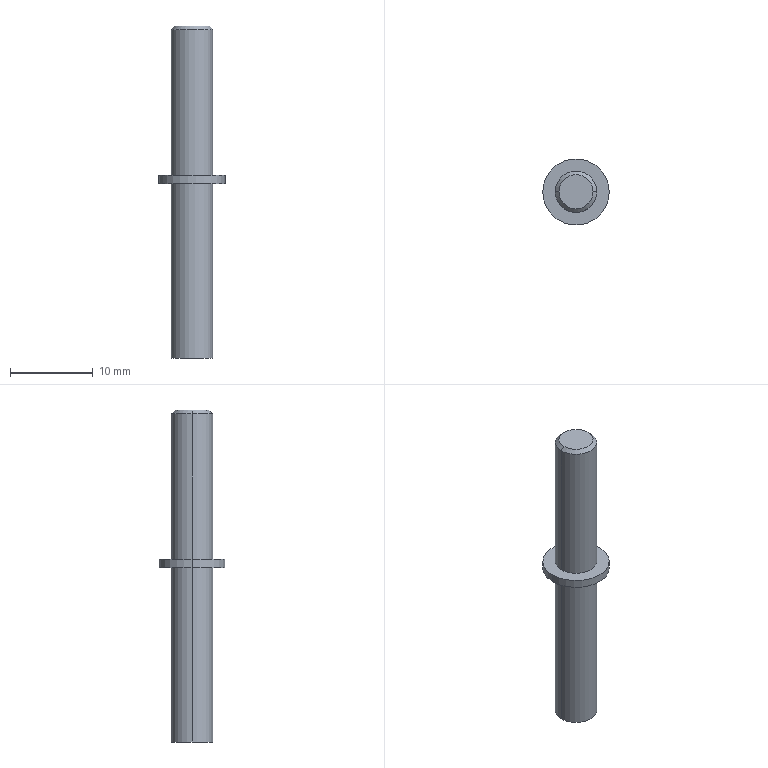Part | SolidWorks | features ICE 2, 3DProfileFeature 1, Extrusion 1, HoleWzd 1, StudWizard 1 | 1 solid | 16 faces | box 8 x 8 x 40 mm | volume 765.722 mm3 | cylinder 8 | cone 4 | plane 4 | commonest cylinder face diameters 5 x4 2.5 x2 8 x2
STEP:
#1=CARTESIAN_POINT('',(0.,0.,-10.549));
#2=VERTEX_POINT('',#1);
#3=CARTESIAN_POINT('',(-1.25,0.,-11.3));
#4=VERTEX_POINT('',#3);
#5=CARTESIAN_POINT('',(-1.25,0.,-11.3));
#6=DIRECTION('',(-0.8572,0.,-0.515));
#7=VECTOR('',#6,1000.);
#8=LINE('',#5,#7);
#9=EDGE_CURVE('',#2,#4,#8,.T.);
#10=ORIENTED_EDGE('',*,*,#9,.F.);
#11=CARTESIAN_POINT('',(1.25,0.,-11.3));
#12=VERTEX_POINT('',#11);
#13=CARTESIAN_POINT('',(1.25,0.,-11.3));
#14=DIRECTION('',(0.8572,0.,-0.515));
#15=VECTOR('',#14,1000.);
#16=LINE('',#13,#15);
#17=EDGE_CURVE('',#2,#12,#16,.T.);
#18=ORIENTED_EDGE('',*,*,#17,.T.);
#19=CARTESIAN_POINT('',(0.,0.,-11.3));
#20=DIRECTION('',(0.,0.,-1.));
#21=DIRECTION('',(-1.,0.,0.));
#22=AXIS2_PLACEMENT_3D('',#19,#20,#21);
#23=CIRCLE('',#22,1.25);
#24=EDGE_CURVE('',#12,#4,#23,.T.);
#25=ORIENTED_EDGE('',*,*,#24,.T.);
#26=EDGE_LOOP('',(#10,#18,#25));
#27=FACE_OUTER_BOUND('',#26,.T.);
#28=CARTESIAN_POINT('',(0.,0.,-11.3));
#29=DIRECTION('',(0.,0.,-1.));
#30=DIRECTION('',(-1.,0.,0.));
#31=AXIS2_PLACEMENT_3D('',#28,#29,#30);
#32=CONICAL_SURFACE('',#31,1.25,1.03);
#33=ADVANCED_FACE('',(#27),#32,.F.);
#34=ORIENTED_EDGE('',*,*,#24,.F.);
#35=CARTESIAN_POINT('',(1.25,0.,-21.));
#36=VERTEX_POINT('',#35);
#37=CARTESIAN_POINT('',(1.25,0.,-21.3));
#38=DIRECTION('',(0.,0.,-1.));
#39=VECTOR('',#38,1000.);
#40=LINE('',#37,#39);
#41=EDGE_CURVE('',#12,#36,#40,.T.);
#42=ORIENTED_EDGE('',*,*,#41,.T.);
#43=CARTESIAN_POINT('',(-1.25,0.,-21.));
#44=VERTEX_POINT('',#43);
#45=CARTESIAN_POINT('',(0.,0.,-21.));
#46=DIRECTION('',(0.,0.,1.));
#47=DIRECTION('',(1.,0.,0.));
#48=AXIS2_PLACEMENT_3D('',#45,#46,#47);
#49=CIRCLE('',#48,1.25);
#50=EDGE_CURVE('',#44,#36,#49,.T.);
#51=ORIENTED_EDGE('',*,*,#50,.F.);
#52=CARTESIAN_POINT('',(-1.25,0.,-21.3));
#53=DIRECTION('',(0.,0.,-1.));
#54=VECTOR('',#53,1000.);
#55=LINE('',#52,#54);
#56=EDGE_CURVE('',#4,#44,#55,.T.);
#57=ORIENTED_EDGE('',*,*,#56,.F.);
#58=EDGE_LOOP('',(#34,#42,#51,#57));
#59=FACE_OUTER_BOUND('',#58,.T.);
#60=CARTESIAN_POINT('',(0.,0.,-21.3));
#61=DIRECTION('',(0.,0.,-1.));
#62=DIRECTION('',(-1.,0.,0.));
#63=AXIS2_PLACEMENT_3D('',#60,#61,#62);
#64=CYLINDRICAL_SURFACE('',#63,1.25);
#65=ADVANCED_FACE('',(#59),#64,.F.);
#66=CARTESIAN_POINT('',(-2.055,0.,19.));
#67=VERTEX_POINT('',#66);
#68=CARTESIAN_POINT('',(2.055,0.,19.));
#69=VERTEX_POINT('',#68);
#70=CARTESIAN_POINT('',(0.,0.,19.));
#71=DIRECTION('',(0.,0.,-1.));
#72=DIRECTION('',(-1.,0.,0.));
#73=AXIS2_PLACEMENT_3D('',#70,#71,#72);
#74=CIRCLE('',#73,2.055);
#75=EDGE_CURVE('',#67,#69,#74,.T.);
#76=ORIENTED_EDGE('',*,*,#75,.T.);
#77=CARTESIAN_POINT('',(2.5,0.,18.555));
#78=VERTEX_POINT('',#77);
#79=CARTESIAN_POINT('',(2.055,0.,19.));
#80=DIRECTION('',(0.7071,0.,-0.7071));
#81=VECTOR('',#80,1000.);
#82=LINE('',#79,#81);
#83=EDGE_CURVE('',#69,#78,#82,.T.);
#84=ORIENTED_EDGE('',*,*,#83,.T.);
#85=CARTESIAN_POINT('',(-2.5,0.,18.555));
#86=VERTEX_POINT('',#85);
#87=CARTESIAN_POINT('',(0.,0.,18.555));
#88=DIRECTION('',(0.,0.,-1.));
#89=DIRECTION('',(-1.,0.,0.));
#90=AXIS2_PLACEMENT_3D('',#87,#88,#89);
#91=CIRCLE('',#90,2.5);
#92=EDGE_CURVE('',#86,#78,#91,.T.);
#93=ORIENTED_EDGE('',*,*,#92,.F.);
#94=CARTESIAN_POINT('',(-2.055,0.,19.));
#95=DIRECTION('',(-0.7071,0.,-0.7071));
#96=VECTOR('',#95,1000.);
#97=LINE('',#94,#96);
#98=EDGE_CURVE('',#67,#86,#97,.T.);
#99=ORIENTED_EDGE('',*,*,#98,.F.);
#100=EDGE_LOOP('',(#76,#84,#93,#99));
#101=FACE_OUTER_BOUND('',#100,.T.);
#102=CARTESIAN_POINT('',(0.,0.,19.));
#103=DIRECTION('',(0.,0.,-1.));
#104=DIRECTION('',(-1.,0.,0.));
#105=AXIS2_PLACEMENT_3D('',#102,#103,#104);
#106=CONICAL_SURFACE('',#105,2.055,0.7854);
#107=ADVANCED_FACE('',(#101),#106,.T.);
#108=ORIENTED_EDGE('',*,*,#92,.T.);
#109=CARTESIAN_POINT('',(2.5,0.,1.));
#110=VERTEX_POINT('',#109);
#111=CARTESIAN_POINT('',(2.5,0.,19.));
#112=DIRECTION('',(0.,0.,-1.));
#113=VECTOR('',#112,1000.);
#114=LINE('',#111,#113);
#115=EDGE_CURVE('',#78,#110,#114,.T.);
#116=ORIENTED_EDGE('',*,*,#115,.T.);
#117=CARTESIAN_POINT('',(-2.5,0.,1.));
#118=VERTEX_POINT('',#117);
#119=CARTESIAN_POINT('',(0.,0.,1.));
#120=DIRECTION('',(0.,0.,1.));
#121=DIRECTION('',(1.,0.,0.));
#122=AXIS2_PLACEMENT_3D('',#119,#120,#121);
#123=CIRCLE('',#122,2.5);
#124=EDGE_CURVE('',#110,#118,#123,.T.);
#125=ORIENTED_EDGE('',*,*,#124,.T.);
#126=CARTESIAN_POINT('',(-2.5,0.,19.));
#127=DIRECTION('',(0.,0.,-1.));
#128=VECTOR('',#127,1000.);
#129=LINE('',#126,#128);
#130=EDGE_CURVE('',#86,#118,#129,.T.);
#131=ORIENTED_EDGE('',*,*,#130,.F.);
#132=EDGE_LOOP('',(#108,#116,#125,#131));
#133=FACE_OUTER_BOUND('',#132,.T.);
#134=CARTESIAN_POINT('',(0.,0.,19.));
#135=DIRECTION('',(0.,0.,-1.));
#136=DIRECTION('',(-1.,0.,0.));
#137=AXIS2_PLACEMENT_3D('',#134,#135,#136);
#138=CYLINDRICAL_SURFACE('',#137,2.5);
#139=ADVANCED_FACE('',(#133),#138,.T.);
#140=CARTESIAN_POINT('',(4.,0.,1.));
#141=VERTEX_POINT('',#140);
#142=CARTESIAN_POINT('',(-4.,0.,1.));
#143=VERTEX_POINT('',#142);
#144=CARTESIAN_POINT('',(0.,0.,1.));
#145=DIRECTION('',(0.,0.,1.));
#146=DIRECTION('',(1.,0.,0.));
#147=AXIS2_PLACEMENT_3D('',#144,#145,#146);
#148=CIRCLE('',#147,4.);
#149=EDGE_CURVE('',#141,#143,#148,.T.);
#150=ORIENTED_EDGE('',*,*,#149,.F.);
#151=CARTESIAN_POINT('',(4.,0.,0.));
#152=VERTEX_POINT('',#151);
#153=CARTESIAN_POINT('',(4.,0.,1.));
#154=DIRECTION('',(0.,0.,-1.));
#155=VECTOR('',#154,1000.);
#156=LINE('',#153,#155);
#157=EDGE_CURVE('',#141,#152,#156,.T.);
#158=ORIENTED_EDGE('',*,*,#157,.T.);
#159=CARTESIAN_POINT('',(-4.,0.,0.));
#160=VERTEX_POINT('',#159);
#161=CARTESIAN_POINT('',(0.,0.,0.));
#162=DIRECTION('',(0.,0.,1.));
#163=DIRECTION('',(1.,0.,0.));
#164=AXIS2_PLACEMENT_3D('',#161,#162,#163);
#165=CIRCLE('',#164,4.);
#166=EDGE_CURVE('',#152,#160,#165,.T.);
#167=ORIENTED_EDGE('',*,*,#166,.T.);
#168=CARTESIAN_POINT('',(-4.,0.,1.));
#169=DIRECTION('',(0.,0.,-1.));
#170=VECTOR('',#169,1000.);
#171=LINE('',#168,#170);
#172=EDGE_CURVE('',#143,#160,#171,.T.);
#173=ORIENTED_EDGE('',*,*,#172,.F.);
#174=EDGE_LOOP('',(#150,#158,#167,#173));
#175=FACE_OUTER_BOUND('',#174,.T.);
#176=CARTESIAN_POINT('',(0.,0.,1.));
#177=DIRECTION('',(0.,0.,-1.));
#178=DIRECTION('',(-1.,0.,0.));
#179=AXIS2_PLACEMENT_3D('',#176,#177,#178);
#180=CYLINDRICAL_SURFACE('',#179,4.);
#181=ADVANCED_FACE('',(#175),#180,.T.);
#182=CARTESIAN_POINT('',(2.5,0.,-21.));
#183=VERTEX_POINT('',#182);
#184=CARTESIAN_POINT('',(-2.5,0.,-21.));
#185=VERTEX_POINT('',#184);
#186=CARTESIAN_POINT('',(0.,0.,-21.));
#187=DIRECTION('',(0.,0.,1.));
#188=DIRECTION('',(1.,0.,0.));
#189=AXIS2_PLACEMENT_3D('',#186,#187,#188);
#190=CIRCLE('',#189,2.5);
#191=EDGE_CURVE('',#183,#185,#190,.T.);
#192=ORIENTED_EDGE('',*,*,#191,.T.);
#193=CARTESIAN_POINT('',(-2.5,0.,0.));
#194=VERTEX_POINT('',#193);
#195=CARTESIAN_POINT('',(-2.5,0.,-21.));
#196=DIRECTION('',(0.,0.,1.));
#197=VECTOR('',#196,1000.);
#198=LINE('',#195,#197);
#199=EDGE_CURVE('',#185,#194,#198,.T.);
#200=ORIENTED_EDGE('',*,*,#199,.T.);
#201=CARTESIAN_POINT('',(2.5,0.,0.));
#202=VERTEX_POINT('',#201);
#203=CARTESIAN_POINT('',(0.,0.,0.));
#204=DIRECTION('',(0.,0.,1.));
#205=DIRECTION('',(1.,0.,0.));
#206=AXIS2_PLACEMENT_3D('',#203,#204,#205);
#207=CIRCLE('',#206,2.5);
#208=EDGE_CURVE('',#202,#194,#207,.T.);
#209=ORIENTED_EDGE('',*,*,#208,.F.);
#210=CARTESIAN_POINT('',(2.5,0.,-21.));
#211=DIRECTION('',(0.,0.,1.));
#212=VECTOR('',#211,1000.);
#213=LINE('',#210,#212);
#214=EDGE_CURVE('',#183,#202,#213,.T.);
#215=ORIENTED_EDGE('',*,*,#214,.F.);
#216=EDGE_LOOP('',(#192,#200,#209,#215));
#217=FACE_OUTER_BOUND('',#216,.T.);
#218=CARTESIAN_POINT('',(0.,0.,-21.));
#219=DIRECTION('',(0.,0.,1.));
#220=DIRECTION('',(1.,0.,0.));
#221=AXIS2_PLACEMENT_3D('',#218,#219,#220);
#222=CYLINDRICAL_SURFACE('',#221,2.5);
#223=ADVANCED_FACE('',(#217),#222,.T.);
#224=ORIENTED_EDGE('',*,*,#199,.F.);
#225=CARTESIAN_POINT('',(0.,0.,-21.));
#226=DIRECTION('',(0.,0.,1.));
#227=DIRECTION('',(1.,0.,0.));
#228=AXIS2_PLACEMENT_3D('',#225,#226,#227);
#229=CIRCLE('',#228,2.5);
#230=EDGE_CURVE('',#185,#183,#229,.T.);
#231=ORIENTED_EDGE('',*,*,#230,.T.);
#232=ORIENTED_EDGE('',*,*,#214,.T.);
#233=CARTESIAN_POINT('',(0.,0.,0.));
#234=DIRECTION('',(0.,0.,1.));
#235=DIRECTION('',(1.,0.,0.));
#236=AXIS2_PLACEMENT_3D('',#233,#234,#235);
#237=CIRCLE('',#236,2.5);
#238=EDGE_CURVE('',#194,#202,#237,.T.);
#239=ORIENTED_EDGE('',*,*,#238,.F.);
#240=EDGE_LOOP('',(#224,#231,#232,#239));
#241=FACE_OUTER_BOUND('',#240,.T.);
#242=CARTESIAN_POINT('',(0.,0.,-21.));
#243=DIRECTION('',(0.,0.,1.));
#244=DIRECTION('',(1.,0.,0.));
#245=AXIS2_PLACEMENT_3D('',#242,#243,#244);
#246=CYLINDRICAL_SURFACE('',#245,2.5);
#247=ADVANCED_FACE('',(#241),#246,.T.);
#248=ORIENTED_EDGE('',*,*,#50,.T.);
#249=CARTESIAN_POINT('',(0.,0.,-21.));
#250=DIRECTION('',(0.,0.,1.));
#251=DIRECTION('',(1.,0.,0.));
#252=AXIS2_PLACEMENT_3D('',#249,#250,#251);
#253=CIRCLE('',#252,1.25);
#254=EDGE_CURVE('',#36,#44,#253,.T.);
#255=ORIENTED_EDGE('',*,*,#254,.T.);
#256=EDGE_LOOP('',(#248,#255));
#257=FACE_BOUND('',#256,.T.);
#258=ORIENTED_EDGE('',*,*,#191,.F.);
#259=ORIENTED_EDGE('',*,*,#230,.F.);
#260=EDGE_LOOP('',(#258,#259));
#261=FACE_OUTER_BOUND('',#260,.T.);
#262=CARTESIAN_POINT('',(0.,0.,-21.));
#263=DIRECTION('',(0.,0.,1.));
#264=DIRECTION('',(1.,0.,0.));
#265=AXIS2_PLACEMENT_3D('',#262,#263,#264);
#266=PLANE('',#265);
#267=ADVANCED_FACE('',(#257,#261),#266,.F.);
#268=ORIENTED_EDGE('',*,*,#157,.F.);
#269=CARTESIAN_POINT('',(0.,0.,1.));
#270=DIRECTION('',(0.,0.,1.));
#271=DIRECTION('',(1.,0.,0.));
#272=AXIS2_PLACEMENT_3D('',#269,#270,#271);
#273=CIRCLE('',#272,4.);
#274=EDGE_CURVE('',#143,#141,#273,.T.);
#275=ORIENTED_EDGE('',*,*,#274,.F.);
#276=ORIENTED_EDGE('',*,*,#172,.T.);
#277=CARTESIAN_POINT('',(0.,0.,0.));
#278=DIRECTION('',(0.,0.,1.));
#279=DIRECTION('',(1.,0.,0.));
#280=AXIS2_PLACEMENT_3D('',#277,#278,#279);
#281=CIRCLE('',#280,4.);
#282=EDGE_CURVE('',#160,#152,#281,.T.);
#283=ORIENTED_EDGE('',*,*,#282,.T.);
#284=EDGE_LOOP('',(#268,#275,#276,#283));
#285=FACE_OUTER_BOUND('',#284,.T.);
#286=CARTESIAN_POINT('',(0.,0.,1.));
#287=DIRECTION('',(0.,0.,-1.));
#288=DIRECTION('',(-1.,0.,0.));
#289=AXIS2_PLACEMENT_3D('',#286,#287,#288);
#290=CYLINDRICAL_SURFACE('',#289,4.);
#291=ADVANCED_FACE('',(#285),#290,.T.);
#292=CARTESIAN_POINT('',(0.,0.,1.));
#293=DIRECTION('',(0.,0.,1.));
#294=DIRECTION('',(1.,0.,0.));
#295=AXIS2_PLACEMENT_3D('',#292,#293,#294);
#296=CIRCLE('',#295,2.5);
#297=EDGE_CURVE('',#118,#110,#296,.T.);
#298=ORIENTED_EDGE('',*,*,#297,.F.);
#299=ORIENTED_EDGE('',*,*,#124,.F.);
#300=EDGE_LOOP('',(#298,#299));
#301=FACE_BOUND('',#300,.T.);
#302=ORIENTED_EDGE('',*,*,#274,.T.);
#303=ORIENTED_EDGE('',*,*,#149,.T.);
#304=EDGE_LOOP('',(#302,#303));
#305=FACE_OUTER_BOUND('',#304,.T.);
#306=CARTESIAN_POINT('',(0.,0.,1.));
#307=DIRECTION('',(0.,0.,1.));
#308=DIRECTION('',(1.,0.,0.));
#309=AXIS2_PLACEMENT_3D('',#306,#307,#308);
#310=PLANE('',#309);
#311=ADVANCED_FACE('',(#301,#305),#310,.T.);
#312=ORIENTED_EDGE('',*,*,#208,.T.);
#313=ORIENTED_EDGE('',*,*,#238,.T.);
#314=EDGE_LOOP('',(#312,#313));
#315=FACE_BOUND('',#314,.T.);
#316=ORIENTED_EDGE('',*,*,#282,.F.);
#317=ORIENTED_EDGE('',*,*,#166,.F.);
#318=EDGE_LOOP('',(#316,#317));
#319=FACE_OUTER_BOUND('',#318,.T.);
#320=CARTESIAN_POINT('',(0.,0.,0.));
#321=DIRECTION('',(0.,0.,1.));
#322=DIRECTION('',(1.,0.,0.));
#323=AXIS2_PLACEMENT_3D('',#320,#321,#322);
#324=PLANE('',#323);
#325=ADVANCED_FACE('',(#315,#319),#324,.F.);
#326=ORIENTED_EDGE('',*,*,#115,.F.);
#327=CARTESIAN_POINT('',(0.,0.,18.555));
#328=DIRECTION('',(0.,0.,-1.));
#329=DIRECTION('',(-1.,0.,0.));
#330=AXIS2_PLACEMENT_3D('',#327,#328,#329);
#331=CIRCLE('',#330,2.5);
#332=EDGE_CURVE('',#78,#86,#331,.T.);
#333=ORIENTED_EDGE('',*,*,#332,.T.);
#334=ORIENTED_EDGE('',*,*,#130,.T.);
#335=ORIENTED_EDGE('',*,*,#297,.T.);
#336=EDGE_LOOP('',(#326,#333,#334,#335));
#337=FACE_OUTER_BOUND('',#336,.T.);
#338=CARTESIAN_POINT('',(0.,0.,19.));
#339=DIRECTION('',(0.,0.,-1.));
#340=DIRECTION('',(-1.,0.,0.));
#341=AXIS2_PLACEMENT_3D('',#338,#339,#340);
#342=CYLINDRICAL_SURFACE('',#341,2.5);
#343=ADVANCED_FACE('',(#337),#342,.T.);
#344=ORIENTED_EDGE('',*,*,#83,.F.);
#345=CARTESIAN_POINT('',(0.,0.,19.));
#346=DIRECTION('',(0.,0.,-1.));
#347=DIRECTION('',(-1.,0.,0.));
#348=AXIS2_PLACEMENT_3D('',#345,#346,#347);
#349=CIRCLE('',#348,2.055);
#350=EDGE_CURVE('',#69,#67,#349,.T.);
#351=ORIENTED_EDGE('',*,*,#350,.T.);
#352=ORIENTED_EDGE('',*,*,#98,.T.);
#353=ORIENTED_EDGE('',*,*,#332,.F.);
#354=EDGE_LOOP('',(#344,#351,#352,#353));
#355=FACE_OUTER_BOUND('',#354,.T.);
#356=CARTESIAN_POINT('',(0.,0.,19.));
#357=DIRECTION('',(0.,0.,-1.));
#358=DIRECTION('',(-1.,0.,0.));
#359=AXIS2_PLACEMENT_3D('',#356,#357,#358);
#360=CONICAL_SURFACE('',#359,2.055,0.7854);
#361=ADVANCED_FACE('',(#355),#360,.T.);
#362=ORIENTED_EDGE('',*,*,#75,.F.);
#363=ORIENTED_EDGE('',*,*,#350,.F.);
#364=EDGE_LOOP('',(#362,#363));
#365=FACE_OUTER_BOUND('',#364,.T.);
#366=CARTESIAN_POINT('',(0.,0.,19.));
#367=DIRECTION('',(0.,0.,1.));
#368=DIRECTION('',(1.,0.,0.));
#369=AXIS2_PLACEMENT_3D('',#366,#367,#368);
#370=PLANE('',#369);
#371=ADVANCED_FACE('',(#365),#370,.T.);
#372=ORIENTED_EDGE('',*,*,#41,.F.);
#373=CARTESIAN_POINT('',(0.,0.,-11.3));
#374=DIRECTION('',(0.,0.,-1.));
#375=DIRECTION('',(-1.,0.,0.));
#376=AXIS2_PLACEMENT_3D('',#373,#374,#375);
#377=CIRCLE('',#376,1.25);
#378=EDGE_CURVE('',#4,#12,#377,.T.);
#379=ORIENTED_EDGE('',*,*,#378,.F.);
#380=ORIENTED_EDGE('',*,*,#56,.T.);
#381=ORIENTED_EDGE('',*,*,#254,.F.);
#382=EDGE_LOOP('',(#372,#379,#380,#381));
#383=FACE_OUTER_BOUND('',#382,.T.);
#384=CARTESIAN_POINT('',(0.,0.,-21.3));
#385=DIRECTION('',(0.,0.,-1.));
#386=DIRECTION('',(-1.,0.,0.));
#387=AXIS2_PLACEMENT_3D('',#384,#385,#386);
#388=CYLINDRICAL_SURFACE('',#387,1.25);
#389=ADVANCED_FACE('',(#383),#388,.F.);
#390=ORIENTED_EDGE('',*,*,#17,.F.);
#391=ORIENTED_EDGE('',*,*,#9,.T.);
#392=ORIENTED_EDGE('',*,*,#378,.T.);
#393=EDGE_LOOP('',(#390,#391,#392));
#394=FACE_OUTER_BOUND('',#393,.T.);
#395=CARTESIAN_POINT('',(0.,0.,-11.3));
#396=DIRECTION('',(0.,0.,-1.));
#397=DIRECTION('',(-1.,0.,0.));
#398=AXIS2_PLACEMENT_3D('',#395,#396,#397);
#399=CONICAL_SURFACE('',#398,1.25,1.03);
#400=ADVANCED_FACE('',(#394),#399,.F.);
#401=CLOSED_SHELL('',(#33,#65,#107,#139,#181,#223,#247,#267,#291,#311,#325,#343,#361,#371,#389,#400));
#402=MANIFOLD_SOLID_BREP('',#401);
#403=CARTESIAN_POINT('',(0.,0.,0.));
#404=DIRECTION('',(0.,0.,1.));
#405=DIRECTION('',(1.,0.,0.));
#406=AXIS2_PLACEMENT_3D('',#403,#404,#405);
#407=(LENGTH_UNIT()NAMED_UNIT(*)SI_UNIT(.MILLI.,.METRE.));
#408=UNCERTAINTY_MEASURE_WITH_UNIT(LENGTH_MEASURE(0.00001),#407,'','');
#409=(NAMED_UNIT(*)PLANE_ANGLE_UNIT()SI_UNIT($,.RADIAN.));
#410=(NAMED_UNIT(*)SI_UNIT($,.STERADIAN.)SOLID_ANGLE_UNIT());
#411=(GEOMETRIC_REPRESENTATION_CONTEXT(3)GLOBAL_UNCERTAINTY_ASSIGNED_CONTEXT((#408))GLOBAL_UNIT_ASSIGNED_CONTEXT((#407,#409,#410))REPRESENTATION_CONTEXT('',''));
#412=ADVANCED_BREP_SHAPE_REPRESENTATION('',(#402,#406),#411);